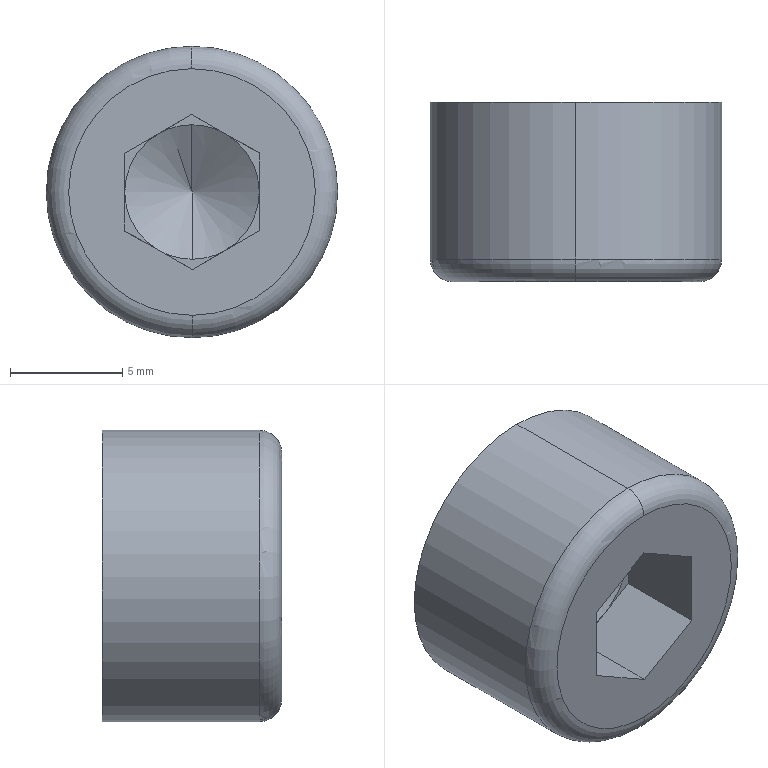Part | SolidWorks | features BaseBody 1 | 1 solid | 20 faces | box 13 x 8 x 13 mm | volume 912.363 mm3 | plane 14 | cone 2 | torus 2 | cylinder 2 | commonest cylinder face diameters 13 x2
STEP:
#1=CARTESIAN_POINT('',(-441.153,-26.768,349.211));
#2=VERTEX_POINT('',#1);
#3=CARTESIAN_POINT('',(-441.142,-28.5,346.211));
#4=VERTEX_POINT('',#3);
#5=CARTESIAN_POINT('',(-441.147,-27.651,347.681));
#6=DIRECTION('',(0.003096,-0.5,-0.866));
#7=VECTOR('',#6,1000.);
#8=LINE('',#5,#7);
#9=EDGE_CURVE('',#2,#4,#8,.T.);
#10=ORIENTED_EDGE('',*,*,#9,.F.);
#11=CARTESIAN_POINT('',(-441.163,-28.5,352.211));
#12=VERTEX_POINT('',#11);
#13=CARTESIAN_POINT('',(-441.158,-27.651,350.741));
#14=DIRECTION('',(-0.003096,-0.5,0.866));
#15=VECTOR('',#14,1000.);
#16=LINE('',#13,#15);
#17=EDGE_CURVE('',#2,#12,#16,.T.);
#18=ORIENTED_EDGE('',*,*,#17,.T.);
#19=CARTESIAN_POINT('',(-442.662,-28.5,351.804));
#20=VERTEX_POINT('',#19);
#21=CARTESIAN_POINT('',(-441.153,-28.5,349.211));
#22=DIRECTION('',(0.,1.,0.));
#23=DIRECTION('',(-0.003575,0.,1.));
#24=AXIS2_PLACEMENT_3D('',#21,#22,#23);
#25=CIRCLE('',#24,3.);
#26=EDGE_CURVE('',#20,#12,#25,.T.);
#27=ORIENTED_EDGE('',*,*,#26,.F.);
#28=CARTESIAN_POINT('',(-444.153,-28.5,349.2));
#29=VERTEX_POINT('',#28);
#30=CARTESIAN_POINT('',(-441.153,-28.5,349.211));
#31=DIRECTION('',(0.,1.,0.));
#32=DIRECTION('',(-1.,0.,-0.003575));
#33=AXIS2_PLACEMENT_3D('',#30,#31,#32);
#34=CIRCLE('',#33,3.);
#35=EDGE_CURVE('',#29,#20,#34,.T.);
#36=ORIENTED_EDGE('',*,*,#35,.F.);
#37=CARTESIAN_POINT('',(-442.643,-28.5,346.608));
#38=VERTEX_POINT('',#37);
#39=CARTESIAN_POINT('',(-441.153,-28.5,349.211));
#40=DIRECTION('',(0.,1.,0.));
#41=DIRECTION('',(-0.4969,0.,-0.8678));
#42=AXIS2_PLACEMENT_3D('',#39,#40,#41);
#43=CIRCLE('',#42,3.);
#44=EDGE_CURVE('',#38,#29,#43,.T.);
#45=ORIENTED_EDGE('',*,*,#44,.F.);
#46=CARTESIAN_POINT('',(-441.153,-28.5,349.211));
#47=DIRECTION('',(0.,1.,0.));
#48=DIRECTION('',(0.5031,0.,-0.8642));
#49=AXIS2_PLACEMENT_3D('',#46,#47,#48);
#50=CIRCLE('',#49,3.);
#51=EDGE_CURVE('',#4,#38,#50,.T.);
#52=ORIENTED_EDGE('',*,*,#51,.F.);
#53=EDGE_LOOP('',(#10,#18,#27,#36,#45,#52));
#54=FACE_OUTER_BOUND('',#53,.T.);
#55=CARTESIAN_POINT('',(-441.153,-27.651,349.211));
#56=DIRECTION('',(0.,-1.,0.));
#57=DIRECTION('',(0.003575,0.,-1.));
#58=AXIS2_PLACEMENT_3D('',#55,#56,#57);
#59=CONICAL_SURFACE('',#58,1.53,1.047);
#60=ADVANCED_FACE('',(#54),#59,.F.);
#61=CARTESIAN_POINT('',(-441.176,-31.5,355.711));
#62=VERTEX_POINT('',#61);
#63=CARTESIAN_POINT('',(-441.129,-31.5,342.711));
#64=VERTEX_POINT('',#63);
#65=CARTESIAN_POINT('',(-441.153,-31.5,349.211));
#66=DIRECTION('',(0.,-1.,0.));
#67=DIRECTION('',(-0.003575,0.,1.));
#68=AXIS2_PLACEMENT_3D('',#65,#66,#67);
#69=CIRCLE('',#68,6.5);
#70=EDGE_CURVE('',#62,#64,#69,.T.);
#71=ORIENTED_EDGE('',*,*,#70,.T.);
#72=CARTESIAN_POINT('',(-441.133,-32.5,343.711));
#73=VERTEX_POINT('',#72);
#74=CARTESIAN_POINT('',(-441.133,-31.5,343.711));
#75=DIRECTION('',(-1.,0.,-0.003575));
#76=DIRECTION('',(-0.003575,0.,1.));
#77=AXIS2_PLACEMENT_3D('',#74,#75,#76);
#78=CIRCLE('',#77,1.);
#79=EDGE_CURVE('',#64,#73,#78,.T.);
#80=ORIENTED_EDGE('',*,*,#79,.T.);
#81=CARTESIAN_POINT('',(-441.172,-32.5,354.711));
#82=VERTEX_POINT('',#81);
#83=CARTESIAN_POINT('',(-441.153,-32.5,349.211));
#84=DIRECTION('',(0.,-1.,0.));
#85=DIRECTION('',(0.003575,0.,-1.));
#86=AXIS2_PLACEMENT_3D('',#83,#84,#85);
#87=CIRCLE('',#86,5.5);
#88=EDGE_CURVE('',#82,#73,#87,.T.);
#89=ORIENTED_EDGE('',*,*,#88,.F.);
#90=CARTESIAN_POINT('',(-441.172,-31.5,354.711));
#91=DIRECTION('',(1.,0.,0.003575));
#92=DIRECTION('',(0.003575,0.,-1.));
#93=AXIS2_PLACEMENT_3D('',#90,#91,#92);
#94=CIRCLE('',#93,1.);
#95=EDGE_CURVE('',#62,#82,#94,.T.);
#96=ORIENTED_EDGE('',*,*,#95,.F.);
#97=EDGE_LOOP('',(#71,#80,#89,#96));
#98=FACE_OUTER_BOUND('',#97,.T.);
#99=CARTESIAN_POINT('',(-441.153,-31.5,349.211));
#100=DIRECTION('',(0.,-1.,0.));
#101=DIRECTION('',(-0.003575,0.,1.));
#102=AXIS2_PLACEMENT_3D('',#99,#100,#101);
#103=TOROIDAL_SURFACE('',#102,5.5,1.);
#104=ADVANCED_FACE('',(#98),#103,.T.);
#105=CARTESIAN_POINT('',(-441.176,-24.5,355.711));
#106=VERTEX_POINT('',#105);
#107=CARTESIAN_POINT('',(-441.129,-24.5,342.711));
#108=VERTEX_POINT('',#107);
#109=CARTESIAN_POINT('',(-441.153,-24.5,349.211));
#110=DIRECTION('',(0.,1.,0.));
#111=DIRECTION('',(0.003575,0.,-1.));
#112=AXIS2_PLACEMENT_3D('',#109,#110,#111);
#113=CIRCLE('',#112,6.5);
#114=EDGE_CURVE('',#106,#108,#113,.T.);
#115=ORIENTED_EDGE('',*,*,#114,.F.);
#116=CARTESIAN_POINT('',(-441.176,-24.5,355.711));
#117=DIRECTION('',(0.,-1.,0.));
#118=VECTOR('',#117,1000.);
#119=LINE('',#116,#118);
#120=EDGE_CURVE('',#106,#62,#119,.T.);
#121=ORIENTED_EDGE('',*,*,#120,.T.);
#122=CARTESIAN_POINT('',(-441.153,-31.5,349.211));
#123=DIRECTION('',(0.,-1.,0.));
#124=DIRECTION('',(-0.003575,0.,1.));
#125=AXIS2_PLACEMENT_3D('',#122,#123,#124);
#126=CIRCLE('',#125,6.5);
#127=EDGE_CURVE('',#64,#62,#126,.T.);
#128=ORIENTED_EDGE('',*,*,#127,.F.);
#129=CARTESIAN_POINT('',(-441.129,-24.5,342.711));
#130=DIRECTION('',(0.,-1.,0.));
#131=VECTOR('',#130,1000.);
#132=LINE('',#129,#131);
#133=EDGE_CURVE('',#108,#64,#132,.T.);
#134=ORIENTED_EDGE('',*,*,#133,.F.);
#135=EDGE_LOOP('',(#115,#121,#128,#134));
#136=FACE_OUTER_BOUND('',#135,.T.);
#137=CARTESIAN_POINT('',(-441.153,-24.5,349.211));
#138=DIRECTION('',(0.,-1.,0.));
#139=DIRECTION('',(0.003575,0.,-1.));
#140=AXIS2_PLACEMENT_3D('',#137,#138,#139);
#141=CYLINDRICAL_SURFACE('',#140,6.5);
#142=ADVANCED_FACE('',(#136),#141,.T.);
#143=CARTESIAN_POINT('',(-441.153,-24.5,349.211));
#144=DIRECTION('',(0.,1.,0.));
#145=DIRECTION('',(0.003575,0.,-1.));
#146=AXIS2_PLACEMENT_3D('',#143,#144,#145);
#147=CIRCLE('',#146,6.5);
#148=EDGE_CURVE('',#108,#106,#147,.T.);
#149=ORIENTED_EDGE('',*,*,#148,.T.);
#150=ORIENTED_EDGE('',*,*,#114,.T.);
#151=EDGE_LOOP('',(#149,#150));
#152=FACE_OUTER_BOUND('',#151,.T.);
#153=CARTESIAN_POINT('',(-441.153,-24.5,349.211));
#154=DIRECTION('',(0.,1.,0.));
#155=DIRECTION('',(1.,0.,0.));
#156=AXIS2_PLACEMENT_3D('',#153,#154,#155);
#157=PLANE('',#156);
#158=ADVANCED_FACE('',(#152),#157,.T.);
#159=ORIENTED_EDGE('',*,*,#120,.F.);
#160=ORIENTED_EDGE('',*,*,#148,.F.);
#161=ORIENTED_EDGE('',*,*,#133,.T.);
#162=ORIENTED_EDGE('',*,*,#70,.F.);
#163=EDGE_LOOP('',(#159,#160,#161,#162));
#164=FACE_OUTER_BOUND('',#163,.T.);
#165=CARTESIAN_POINT('',(-441.153,-24.5,349.211));
#166=DIRECTION('',(0.,-1.,0.));
#167=DIRECTION('',(0.003575,0.,-1.));
#168=AXIS2_PLACEMENT_3D('',#165,#166,#167);
#169=CYLINDRICAL_SURFACE('',#168,6.5);
#170=ADVANCED_FACE('',(#164),#169,.T.);
#171=ORIENTED_EDGE('',*,*,#79,.F.);
#172=ORIENTED_EDGE('',*,*,#127,.T.);
#173=ORIENTED_EDGE('',*,*,#95,.T.);
#174=CARTESIAN_POINT('',(-441.153,-32.5,349.211));
#175=DIRECTION('',(0.,-1.,0.));
#176=DIRECTION('',(0.003575,0.,-1.));
#177=AXIS2_PLACEMENT_3D('',#174,#175,#176);
#178=CIRCLE('',#177,5.5);
#179=EDGE_CURVE('',#73,#82,#178,.T.);
#180=ORIENTED_EDGE('',*,*,#179,.F.);
#181=EDGE_LOOP('',(#171,#172,#173,#180));
#182=FACE_OUTER_BOUND('',#181,.T.);
#183=CARTESIAN_POINT('',(-441.153,-31.5,349.211));
#184=DIRECTION('',(0.,-1.,0.));
#185=DIRECTION('',(-0.003575,0.,1.));
#186=AXIS2_PLACEMENT_3D('',#183,#184,#185);
#187=TOROIDAL_SURFACE('',#186,5.5,1.);
#188=ADVANCED_FACE('',(#182),#187,.T.);
#189=CARTESIAN_POINT('',(-444.146,-32.5,347.468));
#190=VERTEX_POINT('',#189);
#191=CARTESIAN_POINT('',(-444.159,-32.5,350.932));
#192=VERTEX_POINT('',#191);
#193=CARTESIAN_POINT('',(-444.146,-32.5,347.468));
#194=DIRECTION('',(-0.003575,0.,1.));
#195=VECTOR('',#194,1000.);
#196=LINE('',#193,#195);
#197=EDGE_CURVE('',#190,#192,#196,.T.);
#198=ORIENTED_EDGE('',*,*,#197,.T.);
#199=CARTESIAN_POINT('',(-441.165,-32.5,352.675));
#200=VERTEX_POINT('',#199);
#201=CARTESIAN_POINT('',(-444.159,-32.5,350.932));
#202=DIRECTION('',(0.8642,0.,0.5031));
#203=VECTOR('',#202,1000.);
#204=LINE('',#201,#203);
#205=EDGE_CURVE('',#192,#200,#204,.T.);
#206=ORIENTED_EDGE('',*,*,#205,.T.);
#207=CARTESIAN_POINT('',(-438.159,-32.5,350.954));
#208=VERTEX_POINT('',#207);
#209=CARTESIAN_POINT('',(-441.165,-32.5,352.675));
#210=DIRECTION('',(0.8678,0.,-0.4969));
#211=VECTOR('',#210,1000.);
#212=LINE('',#209,#211);
#213=EDGE_CURVE('',#200,#208,#212,.T.);
#214=ORIENTED_EDGE('',*,*,#213,.T.);
#215=CARTESIAN_POINT('',(-438.146,-32.5,347.49));
#216=VERTEX_POINT('',#215);
#217=CARTESIAN_POINT('',(-438.159,-32.5,350.954));
#218=DIRECTION('',(0.003575,0.,-1.));
#219=VECTOR('',#218,1000.);
#220=LINE('',#217,#219);
#221=EDGE_CURVE('',#208,#216,#220,.T.);
#222=ORIENTED_EDGE('',*,*,#221,.T.);
#223=CARTESIAN_POINT('',(-441.14,-32.5,345.747));
#224=VERTEX_POINT('',#223);
#225=CARTESIAN_POINT('',(-438.146,-32.5,347.49));
#226=DIRECTION('',(-0.8642,0.,-0.5031));
#227=VECTOR('',#226,1000.);
#228=LINE('',#225,#227);
#229=EDGE_CURVE('',#216,#224,#228,.T.);
#230=ORIENTED_EDGE('',*,*,#229,.T.);
#231=CARTESIAN_POINT('',(-441.14,-32.5,345.747));
#232=DIRECTION('',(-0.8678,0.,0.4969));
#233=VECTOR('',#232,1000.);
#234=LINE('',#231,#233);
#235=EDGE_CURVE('',#224,#190,#234,.T.);
#236=ORIENTED_EDGE('',*,*,#235,.T.);
#237=EDGE_LOOP('',(#198,#206,#214,#222,#230,#236));
#238=FACE_BOUND('',#237,.T.);
#239=ORIENTED_EDGE('',*,*,#88,.T.);
#240=ORIENTED_EDGE('',*,*,#179,.T.);
#241=EDGE_LOOP('',(#239,#240));
#242=FACE_OUTER_BOUND('',#241,.T.);
#243=CARTESIAN_POINT('',(-441.153,-32.5,349.211));
#244=DIRECTION('',(0.,1.,0.));
#245=DIRECTION('',(1.,0.,0.));
#246=AXIS2_PLACEMENT_3D('',#243,#244,#245);
#247=PLANE('',#246);
#248=ADVANCED_FACE('',(#238,#242),#247,.F.);
#249=CARTESIAN_POINT('',(-444.159,-28.5,350.932));
#250=VERTEX_POINT('',#249);
#251=CARTESIAN_POINT('',(-444.159,-32.5,350.932));
#252=DIRECTION('',(0.,1.,0.));
#253=VECTOR('',#252,1000.);
#254=LINE('',#251,#253);
#255=EDGE_CURVE('',#192,#250,#254,.T.);
#256=ORIENTED_EDGE('',*,*,#255,.F.);
#257=ORIENTED_EDGE('',*,*,#197,.F.);
#258=CARTESIAN_POINT('',(-444.146,-28.5,347.468));
#259=VERTEX_POINT('',#258);
#260=CARTESIAN_POINT('',(-444.146,-32.5,347.468));
#261=DIRECTION('',(0.,1.,0.));
#262=VECTOR('',#261,1000.);
#263=LINE('',#260,#262);
#264=EDGE_CURVE('',#190,#259,#263,.T.);
#265=ORIENTED_EDGE('',*,*,#264,.T.);
#266=CARTESIAN_POINT('',(-444.153,-28.5,349.2));
#267=DIRECTION('',(0.003575,0.,-1.));
#268=VECTOR('',#267,1000.);
#269=LINE('',#266,#268);
#270=EDGE_CURVE('',#29,#259,#269,.T.);
#271=ORIENTED_EDGE('',*,*,#270,.F.);
#272=CARTESIAN_POINT('',(-444.159,-28.5,350.932));
#273=DIRECTION('',(0.003575,0.,-1.));
#274=VECTOR('',#273,1000.);
#275=LINE('',#272,#274);
#276=EDGE_CURVE('',#250,#29,#275,.T.);
#277=ORIENTED_EDGE('',*,*,#276,.F.);
#278=EDGE_LOOP('',(#256,#257,#265,#271,#277));
#279=FACE_OUTER_BOUND('',#278,.T.);
#280=CARTESIAN_POINT('',(-444.146,-28.5,347.468));
#281=DIRECTION('',(1.,0.,0.003575));
#282=DIRECTION('',(0.,-1.,0.));
#283=AXIS2_PLACEMENT_3D('',#280,#281,#282);
#284=PLANE('',#283);
#285=ADVANCED_FACE('',(#279),#284,.T.);
#286=CARTESIAN_POINT('',(-441.165,-28.5,352.675));
#287=VERTEX_POINT('',#286);
#288=CARTESIAN_POINT('',(-441.165,-32.5,352.675));
#289=DIRECTION('',(0.,1.,0.));
#290=VECTOR('',#289,1000.);
#291=LINE('',#288,#290);
#292=EDGE_CURVE('',#200,#287,#291,.T.);
#293=ORIENTED_EDGE('',*,*,#292,.F.);
#294=ORIENTED_EDGE('',*,*,#205,.F.);
#295=ORIENTED_EDGE('',*,*,#255,.T.);
#296=CARTESIAN_POINT('',(-442.662,-28.5,351.804));
#297=DIRECTION('',(-0.8642,0.,-0.5031));
#298=VECTOR('',#297,1000.);
#299=LINE('',#296,#298);
#300=EDGE_CURVE('',#20,#250,#299,.T.);
#301=ORIENTED_EDGE('',*,*,#300,.F.);
#302=CARTESIAN_POINT('',(-441.165,-28.5,352.675));
#303=DIRECTION('',(-0.8642,0.,-0.5031));
#304=VECTOR('',#303,1000.);
#305=LINE('',#302,#304);
#306=EDGE_CURVE('',#287,#20,#305,.T.);
#307=ORIENTED_EDGE('',*,*,#306,.F.);
#308=EDGE_LOOP('',(#293,#294,#295,#301,#307));
#309=FACE_OUTER_BOUND('',#308,.T.);
#310=CARTESIAN_POINT('',(-444.159,-28.5,350.932));
#311=DIRECTION('',(0.5031,0.,-0.8642));
#312=DIRECTION('',(0.,-1.,0.));
#313=AXIS2_PLACEMENT_3D('',#310,#311,#312);
#314=PLANE('',#313);
#315=ADVANCED_FACE('',(#309),#314,.T.);
#316=CARTESIAN_POINT('',(-438.159,-28.5,350.954));
#317=VERTEX_POINT('',#316);
#318=CARTESIAN_POINT('',(-438.159,-32.5,350.954));
#319=DIRECTION('',(0.,1.,0.));
#320=VECTOR('',#319,1000.);
#321=LINE('',#318,#320);
#322=EDGE_CURVE('',#208,#317,#321,.T.);
#323=ORIENTED_EDGE('',*,*,#322,.F.);
#324=ORIENTED_EDGE('',*,*,#213,.F.);
#325=ORIENTED_EDGE('',*,*,#292,.T.);
#326=CARTESIAN_POINT('',(-439.662,-28.5,351.814));
#327=VERTEX_POINT('',#326);
#328=CARTESIAN_POINT('',(-439.662,-28.5,351.814));
#329=DIRECTION('',(-0.8678,0.,0.4969));
#330=VECTOR('',#329,1000.);
#331=LINE('',#328,#330);
#332=EDGE_CURVE('',#327,#287,#331,.T.);
#333=ORIENTED_EDGE('',*,*,#332,.F.);
#334=CARTESIAN_POINT('',(-438.159,-28.5,350.954));
#335=DIRECTION('',(-0.8678,0.,0.4969));
#336=VECTOR('',#335,1000.);
#337=LINE('',#334,#336);
#338=EDGE_CURVE('',#317,#327,#337,.T.);
#339=ORIENTED_EDGE('',*,*,#338,.F.);
#340=EDGE_LOOP('',(#323,#324,#325,#333,#339));
#341=FACE_OUTER_BOUND('',#340,.T.);
#342=CARTESIAN_POINT('',(-441.165,-28.5,352.675));
#343=DIRECTION('',(-0.4969,0.,-0.8678));
#344=DIRECTION('',(-0.8678,0.,0.4969));
#345=AXIS2_PLACEMENT_3D('',#342,#343,#344);
#346=PLANE('',#345);
#347=ADVANCED_FACE('',(#341),#346,.T.);
#348=CARTESIAN_POINT('',(-438.146,-28.5,347.49));
#349=VERTEX_POINT('',#348);
#350=CARTESIAN_POINT('',(-438.146,-28.5,347.49));
#351=DIRECTION('',(0.,-1.,0.));
#352=VECTOR('',#351,1000.);
#353=LINE('',#350,#352);
#354=EDGE_CURVE('',#349,#216,#353,.T.);
#355=ORIENTED_EDGE('',*,*,#354,.T.);
#356=ORIENTED_EDGE('',*,*,#221,.F.);
#357=ORIENTED_EDGE('',*,*,#322,.T.);
#358=CARTESIAN_POINT('',(-438.153,-28.5,349.222));
#359=VERTEX_POINT('',#358);
#360=CARTESIAN_POINT('',(-438.153,-28.5,349.222));
#361=DIRECTION('',(-0.003575,0.,1.));
#362=VECTOR('',#361,1000.);
#363=LINE('',#360,#362);
#364=EDGE_CURVE('',#359,#317,#363,.T.);
#365=ORIENTED_EDGE('',*,*,#364,.F.);
#366=CARTESIAN_POINT('',(-438.146,-28.5,347.49));
#367=DIRECTION('',(-0.003575,0.,1.));
#368=VECTOR('',#367,1000.);
#369=LINE('',#366,#368);
#370=EDGE_CURVE('',#349,#359,#369,.T.);
#371=ORIENTED_EDGE('',*,*,#370,.F.);
#372=EDGE_LOOP('',(#355,#356,#357,#365,#371));
#373=FACE_OUTER_BOUND('',#372,.T.);
#374=CARTESIAN_POINT('',(-438.159,-28.5,350.954));
#375=DIRECTION('',(-1.,0.,-0.003575));
#376=DIRECTION('',(-0.003575,0.,1.));
#377=AXIS2_PLACEMENT_3D('',#374,#375,#376);
#378=PLANE('',#377);
#379=ADVANCED_FACE('',(#373),#378,.T.);
#380=CARTESIAN_POINT('',(-441.14,-28.5,345.747));
#381=VERTEX_POINT('',#380);
#382=CARTESIAN_POINT('',(-441.14,-32.5,345.747));
#383=DIRECTION('',(0.,1.,0.));
#384=VECTOR('',#383,1000.);
#385=LINE('',#382,#384);
#386=EDGE_CURVE('',#224,#381,#385,.T.);
#387=ORIENTED_EDGE('',*,*,#386,.F.);
#388=ORIENTED_EDGE('',*,*,#229,.F.);
#389=ORIENTED_EDGE('',*,*,#354,.F.);
#390=CARTESIAN_POINT('',(-439.643,-28.5,346.618));
#391=VERTEX_POINT('',#390);
#392=CARTESIAN_POINT('',(-439.643,-28.5,346.618));
#393=DIRECTION('',(0.8642,0.,0.5031));
#394=VECTOR('',#393,1000.);
#395=LINE('',#392,#394);
#396=EDGE_CURVE('',#391,#349,#395,.T.);
#397=ORIENTED_EDGE('',*,*,#396,.F.);
#398=CARTESIAN_POINT('',(-441.14,-28.5,345.747));
#399=DIRECTION('',(0.8642,0.,0.5031));
#400=VECTOR('',#399,1000.);
#401=LINE('',#398,#400);
#402=EDGE_CURVE('',#381,#391,#401,.T.);
#403=ORIENTED_EDGE('',*,*,#402,.F.);
#404=EDGE_LOOP('',(#387,#388,#389,#397,#403));
#405=FACE_OUTER_BOUND('',#404,.T.);
#406=CARTESIAN_POINT('',(-438.146,-28.5,347.49));
#407=DIRECTION('',(-0.5031,0.,0.8642));
#408=DIRECTION('',(0.,1.,0.));
#409=AXIS2_PLACEMENT_3D('',#406,#407,#408);
#410=PLANE('',#409);
#411=ADVANCED_FACE('',(#405),#410,.T.);
#412=ORIENTED_EDGE('',*,*,#264,.F.);
#413=ORIENTED_EDGE('',*,*,#235,.F.);
#414=ORIENTED_EDGE('',*,*,#386,.T.);
#415=CARTESIAN_POINT('',(-442.643,-28.5,346.608));
#416=DIRECTION('',(0.8678,0.,-0.4969));
#417=VECTOR('',#416,1000.);
#418=LINE('',#415,#417);
#419=EDGE_CURVE('',#38,#381,#418,.T.);
#420=ORIENTED_EDGE('',*,*,#419,.F.);
#421=CARTESIAN_POINT('',(-444.146,-28.5,347.468));
#422=DIRECTION('',(0.8678,0.,-0.4969));
#423=VECTOR('',#422,1000.);
#424=LINE('',#421,#423);
#425=EDGE_CURVE('',#259,#38,#424,.T.);
#426=ORIENTED_EDGE('',*,*,#425,.F.);
#427=EDGE_LOOP('',(#412,#413,#414,#420,#426));
#428=FACE_OUTER_BOUND('',#427,.T.);
#429=CARTESIAN_POINT('',(-441.14,-28.5,345.747));
#430=DIRECTION('',(0.4969,0.,0.8678));
#431=DIRECTION('',(0.,-1.,0.));
#432=AXIS2_PLACEMENT_3D('',#429,#430,#431);
#433=PLANE('',#432);
#434=ADVANCED_FACE('',(#428),#433,.T.);
#435=ORIENTED_EDGE('',*,*,#425,.T.);
#436=ORIENTED_EDGE('',*,*,#44,.T.);
#437=ORIENTED_EDGE('',*,*,#270,.T.);
#438=EDGE_LOOP('',(#435,#436,#437));
#439=FACE_OUTER_BOUND('',#438,.T.);
#440=CARTESIAN_POINT('',(-441.14,-28.5,345.747));
#441=DIRECTION('',(0.,1.,0.));
#442=DIRECTION('',(1.,0.,0.));
#443=AXIS2_PLACEMENT_3D('',#440,#441,#442);
#444=PLANE('',#443);
#445=ADVANCED_FACE('',(#439),#444,.F.);
#446=ORIENTED_EDGE('',*,*,#276,.T.);
#447=ORIENTED_EDGE('',*,*,#35,.T.);
#448=ORIENTED_EDGE('',*,*,#300,.T.);
#449=EDGE_LOOP('',(#446,#447,#448));
#450=FACE_OUTER_BOUND('',#449,.T.);
#451=CARTESIAN_POINT('',(-441.14,-28.5,345.747));
#452=DIRECTION('',(0.,1.,0.));
#453=DIRECTION('',(1.,0.,0.));
#454=AXIS2_PLACEMENT_3D('',#451,#452,#453);
#455=PLANE('',#454);
#456=ADVANCED_FACE('',(#450),#455,.F.);
#457=ORIENTED_EDGE('',*,*,#306,.T.);
#458=ORIENTED_EDGE('',*,*,#26,.T.);
#459=CARTESIAN_POINT('',(-441.153,-28.5,349.211));
#460=DIRECTION('',(0.,1.,0.));
#461=DIRECTION('',(-0.003575,0.,1.));
#462=AXIS2_PLACEMENT_3D('',#459,#460,#461);
#463=CIRCLE('',#462,3.);
#464=EDGE_CURVE('',#12,#327,#463,.T.);
#465=ORIENTED_EDGE('',*,*,#464,.T.);
#466=ORIENTED_EDGE('',*,*,#332,.T.);
#467=EDGE_LOOP('',(#457,#458,#465,#466));
#468=FACE_OUTER_BOUND('',#467,.T.);
#469=CARTESIAN_POINT('',(-441.14,-28.5,345.747));
#470=DIRECTION('',(0.,1.,0.));
#471=DIRECTION('',(1.,0.,0.));
#472=AXIS2_PLACEMENT_3D('',#469,#470,#471);
#473=PLANE('',#472);
#474=ADVANCED_FACE('',(#468),#473,.F.);
#475=ORIENTED_EDGE('',*,*,#338,.T.);
#476=CARTESIAN_POINT('',(-441.153,-28.5,349.211));
#477=DIRECTION('',(0.,1.,0.));
#478=DIRECTION('',(0.4969,0.,0.8678));
#479=AXIS2_PLACEMENT_3D('',#476,#477,#478);
#480=CIRCLE('',#479,3.);
#481=EDGE_CURVE('',#327,#359,#480,.T.);
#482=ORIENTED_EDGE('',*,*,#481,.T.);
#483=ORIENTED_EDGE('',*,*,#364,.T.);
#484=EDGE_LOOP('',(#475,#482,#483));
#485=FACE_OUTER_BOUND('',#484,.T.);
#486=CARTESIAN_POINT('',(-441.14,-28.5,345.747));
#487=DIRECTION('',(0.,1.,0.));
#488=DIRECTION('',(1.,0.,0.));
#489=AXIS2_PLACEMENT_3D('',#486,#487,#488);
#490=PLANE('',#489);
#491=ADVANCED_FACE('',(#485),#490,.F.);
#492=ORIENTED_EDGE('',*,*,#370,.T.);
#493=CARTESIAN_POINT('',(-441.153,-28.5,349.211));
#494=DIRECTION('',(0.,1.,0.));
#495=DIRECTION('',(1.,0.,0.003575));
#496=AXIS2_PLACEMENT_3D('',#493,#494,#495);
#497=CIRCLE('',#496,3.);
#498=EDGE_CURVE('',#359,#391,#497,.T.);
#499=ORIENTED_EDGE('',*,*,#498,.T.);
#500=ORIENTED_EDGE('',*,*,#396,.T.);
#501=EDGE_LOOP('',(#492,#499,#500));
#502=FACE_OUTER_BOUND('',#501,.T.);
#503=CARTESIAN_POINT('',(-441.14,-28.5,345.747));
#504=DIRECTION('',(0.,1.,0.));
#505=DIRECTION('',(1.,0.,0.));
#506=AXIS2_PLACEMENT_3D('',#503,#504,#505);
#507=PLANE('',#506);
#508=ADVANCED_FACE('',(#502),#507,.F.);
#509=ORIENTED_EDGE('',*,*,#402,.T.);
#510=CARTESIAN_POINT('',(-441.153,-28.5,349.211));
#511=DIRECTION('',(0.,1.,0.));
#512=DIRECTION('',(0.5031,0.,-0.8642));
#513=AXIS2_PLACEMENT_3D('',#510,#511,#512);
#514=CIRCLE('',#513,3.);
#515=EDGE_CURVE('',#391,#4,#514,.T.);
#516=ORIENTED_EDGE('',*,*,#515,.T.);
#517=ORIENTED_EDGE('',*,*,#51,.T.);
#518=ORIENTED_EDGE('',*,*,#419,.T.);
#519=EDGE_LOOP('',(#509,#516,#517,#518));
#520=FACE_OUTER_BOUND('',#519,.T.);
#521=CARTESIAN_POINT('',(-441.14,-28.5,345.747));
#522=DIRECTION('',(0.,1.,0.));
#523=DIRECTION('',(1.,0.,0.));
#524=AXIS2_PLACEMENT_3D('',#521,#522,#523);
#525=PLANE('',#524);
#526=ADVANCED_FACE('',(#520),#525,.F.);
#527=ORIENTED_EDGE('',*,*,#17,.F.);
#528=ORIENTED_EDGE('',*,*,#9,.T.);
#529=ORIENTED_EDGE('',*,*,#515,.F.);
#530=ORIENTED_EDGE('',*,*,#498,.F.);
#531=ORIENTED_EDGE('',*,*,#481,.F.);
#532=ORIENTED_EDGE('',*,*,#464,.F.);
#533=EDGE_LOOP('',(#527,#528,#529,#530,#531,#532));
#534=FACE_OUTER_BOUND('',#533,.T.);
#535=CARTESIAN_POINT('',(-441.153,-27.651,349.211));
#536=DIRECTION('',(0.,-1.,0.));
#537=DIRECTION('',(0.003575,0.,-1.));
#538=AXIS2_PLACEMENT_3D('',#535,#536,#537);
#539=CONICAL_SURFACE('',#538,1.53,1.047);
#540=ADVANCED_FACE('',(#534),#539,.F.);
#541=CLOSED_SHELL('',(#60,#104,#142,#158,#170,#188,#248,#285,#315,#347,#379,#411,#434,#445,#456,#474,#491,#508,#526,#540));
#542=MANIFOLD_SOLID_BREP('',#541);
#543=CARTESIAN_POINT('',(0.,0.,0.));
#544=DIRECTION('',(0.,0.,1.));
#545=DIRECTION('',(1.,0.,0.));
#546=AXIS2_PLACEMENT_3D('',#543,#544,#545);
#547=(LENGTH_UNIT()NAMED_UNIT(*)SI_UNIT(.MILLI.,.METRE.));
#548=UNCERTAINTY_MEASURE_WITH_UNIT(LENGTH_MEASURE(0.00001),#547,'','');
#549=(NAMED_UNIT(*)PLANE_ANGLE_UNIT()SI_UNIT($,.RADIAN.));
#550=(NAMED_UNIT(*)SI_UNIT($,.STERADIAN.)SOLID_ANGLE_UNIT());
#551=(GEOMETRIC_REPRESENTATION_CONTEXT(3)GLOBAL_UNCERTAINTY_ASSIGNED_CONTEXT((#548))GLOBAL_UNIT_ASSIGNED_CONTEXT((#547,#549,#550))REPRESENTATION_CONTEXT('',''));
#552=ADVANCED_BREP_SHAPE_REPRESENTATION('',(#542,#546),#551);